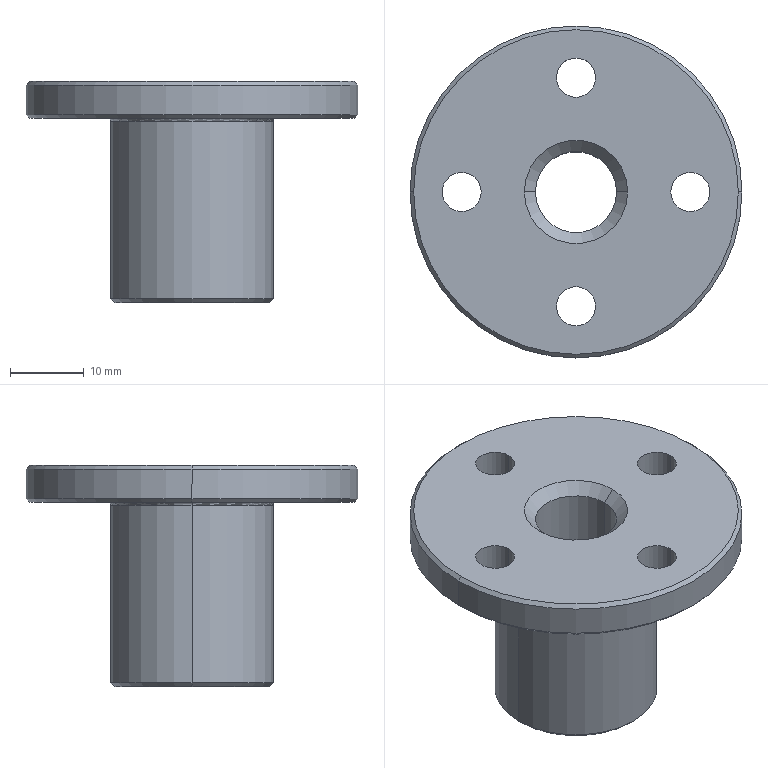Part | STEP file | 001-003-LJL74-d14 | 1 solid | 29 faces | box 45 x 45 x 30 mm | volume 14037 mm3 | cylinder 14 | cone 10 | plane 3 | torus 2 | commonest cylinder face diameters 5.3 x8 11 x2 22 x2 45 x2